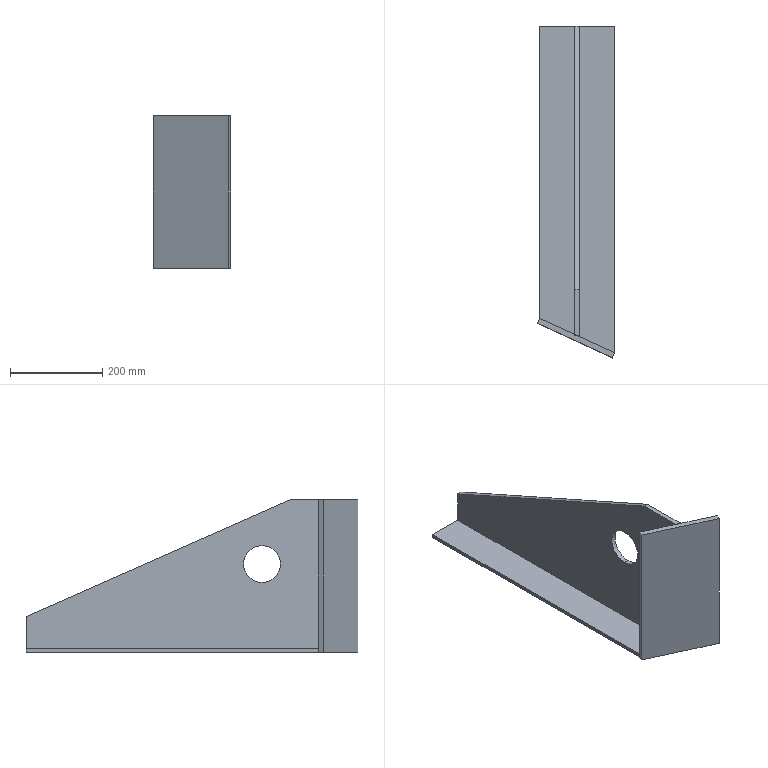Part | STEP file | Edge support_Default<As machined> | 3 solids | 21 faces | box 168.631 x 720.909 x 332 mm | volume 2997743 mm3 | plane 19 | cylinder 2 | commonest cylinder face diameters 80 x2
STEP:
#1=CARTESIAN_POINT('',(0.,0.,0.));
#2=DIRECTION('',(0.,0.,1.));
#3=DIRECTION('',(1.,0.,0.));
#4=AXIS2_PLACEMENT_3D('',#1,#2,#3);
#5=CARTESIAN_POINT('',(-81.815,0.,-4.));
#6=VERTEX_POINT('',#5);
#7=CARTESIAN_POINT('',(-81.815,-635.,-4.));
#8=VERTEX_POINT('',#7);
#9=CARTESIAN_POINT('',(-81.815,-635.,-4.));
#10=DIRECTION('',(0.,-1.,0.));
#11=VECTOR('',#10,1.);
#12=LINE('',#9,#11);
#13=CARTESIAN_POINT('',(-81.815,-635.,4.));
#14=DIRECTION('',(1.,0.,0.));
#15=DIRECTION('',(0.,0.,-1.));
#16=AXIS2_PLACEMENT_3D('',#13,#14,#15);
#17=PLANE('',#16);
#18=CARTESIAN_POINT('',(8.,0.));
#19=DIRECTION('',(0.,-1.));
#20=VECTOR('',#19,1.);
#21=LINE('',#18,#20);
#22=(GEOMETRIC_REPRESENTATION_CONTEXT(2)PARAMETRIC_REPRESENTATION_CONTEXT()REPRESENTATION_CONTEXT('',''));
#23=DEFINITIONAL_REPRESENTATION('',(#21),#22);
#24=PCURVE('',#17,#23);
#25=CARTESIAN_POINT('',(0.,0.,-4.));
#26=DIRECTION('',(0.,0.,-1.));
#27=DIRECTION('',(-1.,0.,0.));
#28=AXIS2_PLACEMENT_3D('',#25,#26,#27);
#29=PLANE('',#28);
#30=CARTESIAN_POINT('',(81.815,-635.));
#31=DIRECTION('',(0.,-1.));
#32=VECTOR('',#31,1.);
#33=LINE('',#30,#32);
#34=(GEOMETRIC_REPRESENTATION_CONTEXT(2)PARAMETRIC_REPRESENTATION_CONTEXT()REPRESENTATION_CONTEXT('',''));
#35=DEFINITIONAL_REPRESENTATION('',(#33),#34);
#36=PCURVE('',#29,#35);
#37=SURFACE_CURVE('',#12,(#24,#36),.PCURVE_S1.);
#38=EDGE_CURVE('',#6,#8,#37,.T.);
#39=ORIENTED_EDGE('',*,*,#38,.T.);
#40=CARTESIAN_POINT('',(-81.815,-635.,4.));
#41=VERTEX_POINT('',#40);
#42=CARTESIAN_POINT('',(-81.815,-635.,4.));
#43=DIRECTION('',(0.,0.,-1.));
#44=VECTOR('',#43,1.);
#45=LINE('',#42,#44);
#46=CARTESIAN_POINT('',(0.,0.));
#47=DIRECTION('',(1.,0.));
#48=VECTOR('',#47,1.);
#49=LINE('',#46,#48);
#50=(GEOMETRIC_REPRESENTATION_CONTEXT(2)PARAMETRIC_REPRESENTATION_CONTEXT()REPRESENTATION_CONTEXT('',''));
#51=DEFINITIONAL_REPRESENTATION('',(#49),#50);
#52=PCURVE('',#17,#51);
#53=CARTESIAN_POINT('',(81.815,-710.,4.));
#54=DIRECTION('',(0.4167,0.9091,0.));
#55=DIRECTION('',(-0.9091,0.4167,0.));
#56=AXIS2_PLACEMENT_3D('',#53,#54,#55);
#57=PLANE('',#56);
#58=CARTESIAN_POINT('',(180.,0.));
#59=DIRECTION('',(0.,-1.));
#60=VECTOR('',#59,1.);
#61=LINE('',#58,#60);
#62=(GEOMETRIC_REPRESENTATION_CONTEXT(2)PARAMETRIC_REPRESENTATION_CONTEXT()REPRESENTATION_CONTEXT('',''));
#63=DEFINITIONAL_REPRESENTATION('',(#61),#62);
#64=PCURVE('',#57,#63);
#65=SURFACE_CURVE('',#45,(#52,#64),.PCURVE_S1.);
#66=EDGE_CURVE('',#41,#8,#65,.T.);
#67=ORIENTED_EDGE('',*,*,#66,.F.);
#68=CARTESIAN_POINT('',(-81.815,0.,4.));
#69=VERTEX_POINT('',#68);
#70=CARTESIAN_POINT('',(-81.815,-635.,4.));
#71=DIRECTION('',(0.,-1.,0.));
#72=VECTOR('',#71,1.);
#73=LINE('',#70,#72);
#74=CARTESIAN_POINT('',(0.,0.));
#75=DIRECTION('',(0.,-1.));
#76=VECTOR('',#75,1.);
#77=LINE('',#74,#76);
#78=(GEOMETRIC_REPRESENTATION_CONTEXT(2)PARAMETRIC_REPRESENTATION_CONTEXT()REPRESENTATION_CONTEXT('',''));
#79=DEFINITIONAL_REPRESENTATION('',(#77),#78);
#80=PCURVE('',#17,#79);
#81=CARTESIAN_POINT('',(0.,0.,4.));
#82=DIRECTION('',(0.,0.,-1.));
#83=DIRECTION('',(-1.,0.,0.));
#84=AXIS2_PLACEMENT_3D('',#81,#82,#83);
#85=PLANE('',#84);
#86=CARTESIAN_POINT('',(81.815,-635.));
#87=DIRECTION('',(0.,-1.));
#88=VECTOR('',#87,1.);
#89=LINE('',#86,#88);
#90=(GEOMETRIC_REPRESENTATION_CONTEXT(2)PARAMETRIC_REPRESENTATION_CONTEXT()REPRESENTATION_CONTEXT('',''));
#91=DEFINITIONAL_REPRESENTATION('',(#89),#90);
#92=PCURVE('',#85,#91);
#93=SURFACE_CURVE('',#73,(#80,#92),.PCURVE_S1.);
#94=EDGE_CURVE('',#69,#41,#93,.T.);
#95=ORIENTED_EDGE('',*,*,#94,.F.);
#96=CARTESIAN_POINT('',(-81.815,0.,4.));
#97=DIRECTION('',(0.,0.,-1.));
#98=VECTOR('',#97,1.);
#99=LINE('',#96,#98);
#100=CARTESIAN_POINT('',(0.,635.));
#101=DIRECTION('',(1.,0.));
#102=VECTOR('',#101,1.);
#103=LINE('',#100,#102);
#104=(GEOMETRIC_REPRESENTATION_CONTEXT(2)PARAMETRIC_REPRESENTATION_CONTEXT()REPRESENTATION_CONTEXT('',''));
#105=DEFINITIONAL_REPRESENTATION('',(#103),#104);
#106=PCURVE('',#17,#105);
#107=CARTESIAN_POINT('',(-81.815,0.,4.));
#108=DIRECTION('',(0.,-1.,0.));
#109=DIRECTION('',(1.,0.,0.));
#110=AXIS2_PLACEMENT_3D('',#107,#108,#109);
#111=PLANE('',#110);
#112=CARTESIAN_POINT('',(0.,0.));
#113=DIRECTION('',(0.,-1.));
#114=VECTOR('',#113,1.);
#115=LINE('',#112,#114);
#116=(GEOMETRIC_REPRESENTATION_CONTEXT(2)PARAMETRIC_REPRESENTATION_CONTEXT()REPRESENTATION_CONTEXT('',''));
#117=DEFINITIONAL_REPRESENTATION('',(#115),#116);
#118=PCURVE('',#111,#117);
#119=SURFACE_CURVE('',#99,(#106,#118),.PCURVE_S1.);
#120=EDGE_CURVE('',#69,#6,#119,.T.);
#121=ORIENTED_EDGE('',*,*,#120,.T.);
#122=EDGE_LOOP('',(#39,#67,#95,#121));
#123=FACE_BOUND('',#122,.T.);
#124=ADVANCED_FACE('',(#123),#17,.F.);
#125=CARTESIAN_POINT('',(81.815,-710.,-4.));
#126=VERTEX_POINT('',#125);
#127=CARTESIAN_POINT('',(81.815,-710.,-4.));
#128=DIRECTION('',(0.9091,-0.4167,0.));
#129=VECTOR('',#128,1.);
#130=LINE('',#127,#129);
#131=CARTESIAN_POINT('',(0.,-8.));
#132=DIRECTION('',(-1.,0.));
#133=VECTOR('',#132,1.);
#134=LINE('',#131,#133);
#135=(GEOMETRIC_REPRESENTATION_CONTEXT(2)PARAMETRIC_REPRESENTATION_CONTEXT()REPRESENTATION_CONTEXT('',''));
#136=DEFINITIONAL_REPRESENTATION('',(#134),#135);
#137=PCURVE('',#57,#136);
#138=CARTESIAN_POINT('',(-81.815,-710.));
#139=DIRECTION('',(-0.9091,-0.4167));
#140=VECTOR('',#139,1.);
#141=LINE('',#138,#140);
#142=(GEOMETRIC_REPRESENTATION_CONTEXT(2)PARAMETRIC_REPRESENTATION_CONTEXT()REPRESENTATION_CONTEXT('',''));
#143=DEFINITIONAL_REPRESENTATION('',(#141),#142);
#144=PCURVE('',#29,#143);
#145=SURFACE_CURVE('',#130,(#137,#144),.PCURVE_S1.);
#146=EDGE_CURVE('',#8,#126,#145,.T.);
#147=ORIENTED_EDGE('',*,*,#146,.T.);
#148=CARTESIAN_POINT('',(81.815,-710.,4.));
#149=VERTEX_POINT('',#148);
#150=CARTESIAN_POINT('',(81.815,-710.,4.));
#151=DIRECTION('',(0.,0.,-1.));
#152=VECTOR('',#151,1.);
#153=LINE('',#150,#152);
#154=CARTESIAN_POINT('',(0.,0.));
#155=DIRECTION('',(0.,-1.));
#156=VECTOR('',#155,1.);
#157=LINE('',#154,#156);
#158=(GEOMETRIC_REPRESENTATION_CONTEXT(2)PARAMETRIC_REPRESENTATION_CONTEXT()REPRESENTATION_CONTEXT('',''));
#159=DEFINITIONAL_REPRESENTATION('',(#157),#158);
#160=PCURVE('',#57,#159);
#161=CARTESIAN_POINT('',(81.815,0.,4.));
#162=DIRECTION('',(-1.,0.,0.));
#163=DIRECTION('',(0.,0.,1.));
#164=AXIS2_PLACEMENT_3D('',#161,#162,#163);
#165=PLANE('',#164);
#166=CARTESIAN_POINT('',(0.,-710.));
#167=DIRECTION('',(-1.,0.));
#168=VECTOR('',#167,1.);
#169=LINE('',#166,#168);
#170=(GEOMETRIC_REPRESENTATION_CONTEXT(2)PARAMETRIC_REPRESENTATION_CONTEXT()REPRESENTATION_CONTEXT('',''));
#171=DEFINITIONAL_REPRESENTATION('',(#169),#170);
#172=PCURVE('',#165,#171);
#173=SURFACE_CURVE('',#153,(#160,#172),.PCURVE_S1.);
#174=EDGE_CURVE('',#149,#126,#173,.T.);
#175=ORIENTED_EDGE('',*,*,#174,.F.);
#176=CARTESIAN_POINT('',(81.815,-710.,4.));
#177=DIRECTION('',(0.9091,-0.4167,0.));
#178=VECTOR('',#177,1.);
#179=LINE('',#176,#178);
#180=CARTESIAN_POINT('',(0.,0.));
#181=DIRECTION('',(-1.,0.));
#182=VECTOR('',#181,1.);
#183=LINE('',#180,#182);
#184=(GEOMETRIC_REPRESENTATION_CONTEXT(2)PARAMETRIC_REPRESENTATION_CONTEXT()REPRESENTATION_CONTEXT('',''));
#185=DEFINITIONAL_REPRESENTATION('',(#183),#184);
#186=PCURVE('',#57,#185);
#187=CARTESIAN_POINT('',(-81.815,-710.));
#188=DIRECTION('',(-0.9091,-0.4167));
#189=VECTOR('',#188,1.);
#190=LINE('',#187,#189);
#191=(GEOMETRIC_REPRESENTATION_CONTEXT(2)PARAMETRIC_REPRESENTATION_CONTEXT()REPRESENTATION_CONTEXT('',''));
#192=DEFINITIONAL_REPRESENTATION('',(#190),#191);
#193=PCURVE('',#85,#192);
#194=SURFACE_CURVE('',#179,(#186,#193),.PCURVE_S1.);
#195=EDGE_CURVE('',#41,#149,#194,.T.);
#196=ORIENTED_EDGE('',*,*,#195,.F.);
#197=ORIENTED_EDGE('',*,*,#66,.T.);
#198=EDGE_LOOP('',(#147,#175,#196,#197));
#199=FACE_BOUND('',#198,.T.);
#200=ADVANCED_FACE('',(#199),#57,.F.);
#201=CARTESIAN_POINT('',(81.815,0.,-4.));
#202=VERTEX_POINT('',#201);
#203=CARTESIAN_POINT('',(81.815,0.,-4.));
#204=DIRECTION('',(0.,1.,0.));
#205=VECTOR('',#204,1.);
#206=LINE('',#203,#205);
#207=CARTESIAN_POINT('',(-8.,0.));
#208=DIRECTION('',(0.,1.));
#209=VECTOR('',#208,1.);
#210=LINE('',#207,#209);
#211=(GEOMETRIC_REPRESENTATION_CONTEXT(2)PARAMETRIC_REPRESENTATION_CONTEXT()REPRESENTATION_CONTEXT('',''));
#212=DEFINITIONAL_REPRESENTATION('',(#210),#211);
#213=PCURVE('',#165,#212);
#214=CARTESIAN_POINT('',(-81.815,0.));
#215=DIRECTION('',(0.,1.));
#216=VECTOR('',#215,1.);
#217=LINE('',#214,#216);
#218=(GEOMETRIC_REPRESENTATION_CONTEXT(2)PARAMETRIC_REPRESENTATION_CONTEXT()REPRESENTATION_CONTEXT('',''));
#219=DEFINITIONAL_REPRESENTATION('',(#217),#218);
#220=PCURVE('',#29,#219);
#221=SURFACE_CURVE('',#206,(#213,#220),.PCURVE_S1.);
#222=EDGE_CURVE('',#126,#202,#221,.T.);
#223=ORIENTED_EDGE('',*,*,#222,.T.);
#224=CARTESIAN_POINT('',(81.815,0.,4.));
#225=VERTEX_POINT('',#224);
#226=CARTESIAN_POINT('',(81.815,0.,4.));
#227=DIRECTION('',(0.,0.,-1.));
#228=VECTOR('',#227,1.);
#229=LINE('',#226,#228);
#230=CARTESIAN_POINT('',(0.,0.));
#231=DIRECTION('',(-1.,0.));
#232=VECTOR('',#231,1.);
#233=LINE('',#230,#232);
#234=(GEOMETRIC_REPRESENTATION_CONTEXT(2)PARAMETRIC_REPRESENTATION_CONTEXT()REPRESENTATION_CONTEXT('',''));
#235=DEFINITIONAL_REPRESENTATION('',(#233),#234);
#236=PCURVE('',#165,#235);
#237=CARTESIAN_POINT('',(163.631,0.));
#238=DIRECTION('',(0.,-1.));
#239=VECTOR('',#238,1.);
#240=LINE('',#237,#239);
#241=(GEOMETRIC_REPRESENTATION_CONTEXT(2)PARAMETRIC_REPRESENTATION_CONTEXT()REPRESENTATION_CONTEXT('',''));
#242=DEFINITIONAL_REPRESENTATION('',(#240),#241);
#243=PCURVE('',#111,#242);
#244=SURFACE_CURVE('',#229,(#236,#243),.PCURVE_S1.);
#245=EDGE_CURVE('',#225,#202,#244,.T.);
#246=ORIENTED_EDGE('',*,*,#245,.F.);
#247=CARTESIAN_POINT('',(81.815,0.,4.));
#248=DIRECTION('',(0.,1.,0.));
#249=VECTOR('',#248,1.);
#250=LINE('',#247,#249);
#251=CARTESIAN_POINT('',(0.,0.));
#252=DIRECTION('',(0.,1.));
#253=VECTOR('',#252,1.);
#254=LINE('',#251,#253);
#255=(GEOMETRIC_REPRESENTATION_CONTEXT(2)PARAMETRIC_REPRESENTATION_CONTEXT()REPRESENTATION_CONTEXT('',''));
#256=DEFINITIONAL_REPRESENTATION('',(#254),#255);
#257=PCURVE('',#165,#256);
#258=CARTESIAN_POINT('',(-81.815,0.));
#259=DIRECTION('',(0.,1.));
#260=VECTOR('',#259,1.);
#261=LINE('',#258,#260);
#262=(GEOMETRIC_REPRESENTATION_CONTEXT(2)PARAMETRIC_REPRESENTATION_CONTEXT()REPRESENTATION_CONTEXT('',''));
#263=DEFINITIONAL_REPRESENTATION('',(#261),#262);
#264=PCURVE('',#85,#263);
#265=SURFACE_CURVE('',#250,(#257,#264),.PCURVE_S1.);
#266=EDGE_CURVE('',#149,#225,#265,.T.);
#267=ORIENTED_EDGE('',*,*,#266,.F.);
#268=ORIENTED_EDGE('',*,*,#174,.T.);
#269=EDGE_LOOP('',(#223,#246,#267,#268));
#270=FACE_BOUND('',#269,.T.);
#271=ADVANCED_FACE('',(#270),#165,.F.);
#272=CARTESIAN_POINT('',(-81.815,0.,-4.));
#273=DIRECTION('',(-1.,0.,0.));
#274=VECTOR('',#273,1.);
#275=LINE('',#272,#274);
#276=CARTESIAN_POINT('',(0.,-8.));
#277=DIRECTION('',(-1.,0.));
#278=VECTOR('',#277,1.);
#279=LINE('',#276,#278);
#280=(GEOMETRIC_REPRESENTATION_CONTEXT(2)PARAMETRIC_REPRESENTATION_CONTEXT()REPRESENTATION_CONTEXT('',''));
#281=DEFINITIONAL_REPRESENTATION('',(#279),#280);
#282=PCURVE('',#111,#281);
#283=CARTESIAN_POINT('',(81.815,0.));
#284=DIRECTION('',(1.,0.));
#285=VECTOR('',#284,1.);
#286=LINE('',#283,#285);
#287=(GEOMETRIC_REPRESENTATION_CONTEXT(2)PARAMETRIC_REPRESENTATION_CONTEXT()REPRESENTATION_CONTEXT('',''));
#288=DEFINITIONAL_REPRESENTATION('',(#286),#287);
#289=PCURVE('',#29,#288);
#290=SURFACE_CURVE('',#275,(#282,#289),.PCURVE_S1.);
#291=EDGE_CURVE('',#202,#6,#290,.T.);
#292=ORIENTED_EDGE('',*,*,#291,.T.);
#293=ORIENTED_EDGE('',*,*,#120,.F.);
#294=CARTESIAN_POINT('',(-81.815,0.,4.));
#295=DIRECTION('',(-1.,0.,0.));
#296=VECTOR('',#295,1.);
#297=LINE('',#294,#296);
#298=CARTESIAN_POINT('',(0.,0.));
#299=DIRECTION('',(-1.,0.));
#300=VECTOR('',#299,1.);
#301=LINE('',#298,#300);
#302=(GEOMETRIC_REPRESENTATION_CONTEXT(2)PARAMETRIC_REPRESENTATION_CONTEXT()REPRESENTATION_CONTEXT('',''));
#303=DEFINITIONAL_REPRESENTATION('',(#301),#302);
#304=PCURVE('',#111,#303);
#305=CARTESIAN_POINT('',(81.815,0.));
#306=DIRECTION('',(1.,0.));
#307=VECTOR('',#306,1.);
#308=LINE('',#305,#307);
#309=(GEOMETRIC_REPRESENTATION_CONTEXT(2)PARAMETRIC_REPRESENTATION_CONTEXT()REPRESENTATION_CONTEXT('',''));
#310=DEFINITIONAL_REPRESENTATION('',(#308),#309);
#311=PCURVE('',#85,#310);
#312=SURFACE_CURVE('',#297,(#304,#311),.PCURVE_S1.);
#313=EDGE_CURVE('',#225,#69,#312,.T.);
#314=ORIENTED_EDGE('',*,*,#313,.F.);
#315=ORIENTED_EDGE('',*,*,#245,.T.);
#316=EDGE_LOOP('',(#292,#293,#314,#315));
#317=FACE_BOUND('',#316,.T.);
#318=ADVANCED_FACE('',(#317),#111,.F.);
#319=ORIENTED_EDGE('',*,*,#94,.T.);
#320=ORIENTED_EDGE('',*,*,#195,.T.);
#321=ORIENTED_EDGE('',*,*,#266,.T.);
#322=ORIENTED_EDGE('',*,*,#313,.T.);
#323=EDGE_LOOP('',(#319,#320,#321,#322));
#324=FACE_BOUND('',#323,.T.);
#325=ADVANCED_FACE('',(#324),#85,.F.);
#326=ORIENTED_EDGE('',*,*,#38,.F.);
#327=ORIENTED_EDGE('',*,*,#291,.F.);
#328=ORIENTED_EDGE('',*,*,#222,.F.);
#329=ORIENTED_EDGE('',*,*,#146,.F.);
#330=EDGE_LOOP('',(#326,#327,#328,#329));
#331=FACE_BOUND('',#330,.T.);
#332=ADVANCED_FACE('',(#331),#29,.T.);
#333=CLOSED_SHELL('',(#124,#200,#271,#318,#325,#332));
#334=MANIFOLD_SOLID_BREP('',#333);
#335=CARTESIAN_POINT('',(-81.815,-635.,-4.));
#336=VERTEX_POINT('',#335);
#337=CARTESIAN_POINT('',(-86.815,-645.909,-4.));
#338=VERTEX_POINT('',#337);
#339=CARTESIAN_POINT('',(-86.815,-645.909,-4.));
#340=DIRECTION('',(-0.4167,-0.9091,0.));
#341=VECTOR('',#340,1.);
#342=LINE('',#339,#341);
#343=CARTESIAN_POINT('',(-86.815,-645.909,328.));
#344=DIRECTION('',(0.9091,-0.4167,0.));
#345=DIRECTION('',(0.4167,0.9091,0.));
#346=AXIS2_PLACEMENT_3D('',#343,#344,#345);
#347=PLANE('',#346);
#348=CARTESIAN_POINT('',(0.,-332.));
#349=DIRECTION('',(-1.,0.));
#350=VECTOR('',#349,1.);
#351=LINE('',#348,#350);
#352=(GEOMETRIC_REPRESENTATION_CONTEXT(2)PARAMETRIC_REPRESENTATION_CONTEXT()REPRESENTATION_CONTEXT('',''));
#353=DEFINITIONAL_REPRESENTATION('',(#351),#352);
#354=PCURVE('',#347,#353);
#355=CARTESIAN_POINT('',(0.,0.,-4.));
#356=DIRECTION('',(0.,0.,-1.));
#357=DIRECTION('',(-1.,0.,0.));
#358=AXIS2_PLACEMENT_3D('',#355,#356,#357);
#359=PLANE('',#358);
#360=CARTESIAN_POINT('',(86.815,-645.909));
#361=DIRECTION('',(0.4167,-0.9091));
#362=VECTOR('',#361,1.);
#363=LINE('',#360,#362);
#364=(GEOMETRIC_REPRESENTATION_CONTEXT(2)PARAMETRIC_REPRESENTATION_CONTEXT()REPRESENTATION_CONTEXT('',''));
#365=DEFINITIONAL_REPRESENTATION('',(#363),#364);
#366=PCURVE('',#359,#365);
#367=SURFACE_CURVE('',#342,(#354,#366),.PCURVE_S1.);
#368=EDGE_CURVE('',#336,#338,#367,.T.);
#369=ORIENTED_EDGE('',*,*,#368,.T.);
#370=CARTESIAN_POINT('',(-86.815,-645.909,328.));
#371=VERTEX_POINT('',#370);
#372=CARTESIAN_POINT('',(-86.815,-645.909,328.));
#373=DIRECTION('',(0.,0.,-1.));
#374=VECTOR('',#373,1.);
#375=LINE('',#372,#374);
#376=CARTESIAN_POINT('',(0.,0.));
#377=DIRECTION('',(0.,-1.));
#378=VECTOR('',#377,1.);
#379=LINE('',#376,#378);
#380=(GEOMETRIC_REPRESENTATION_CONTEXT(2)PARAMETRIC_REPRESENTATION_CONTEXT()REPRESENTATION_CONTEXT('',''));
#381=DEFINITIONAL_REPRESENTATION('',(#379),#380);
#382=PCURVE('',#347,#381);
#383=CARTESIAN_POINT('',(76.815,-720.909,328.));
#384=DIRECTION('',(0.4167,0.9091,0.));
#385=DIRECTION('',(-0.9091,0.4167,0.));
#386=AXIS2_PLACEMENT_3D('',#383,#384,#385);
#387=PLANE('',#386);
#388=CARTESIAN_POINT('',(180.,0.));
#389=DIRECTION('',(0.,-1.));
#390=VECTOR('',#389,1.);
#391=LINE('',#388,#390);
#392=(GEOMETRIC_REPRESENTATION_CONTEXT(2)PARAMETRIC_REPRESENTATION_CONTEXT()REPRESENTATION_CONTEXT('',''));
#393=DEFINITIONAL_REPRESENTATION('',(#391),#392);
#394=PCURVE('',#387,#393);
#395=SURFACE_CURVE('',#375,(#382,#394),.PCURVE_S1.);
#396=EDGE_CURVE('',#371,#338,#395,.T.);
#397=ORIENTED_EDGE('',*,*,#396,.F.);
#398=CARTESIAN_POINT('',(-81.815,-635.,328.));
#399=VERTEX_POINT('',#398);
#400=CARTESIAN_POINT('',(-86.815,-645.909,328.));
#401=DIRECTION('',(-0.4167,-0.9091,0.));
#402=VECTOR('',#401,1.);
#403=LINE('',#400,#402);
#404=CARTESIAN_POINT('',(0.,0.));
#405=DIRECTION('',(-1.,0.));
#406=VECTOR('',#405,1.);
#407=LINE('',#404,#406);
#408=(GEOMETRIC_REPRESENTATION_CONTEXT(2)PARAMETRIC_REPRESENTATION_CONTEXT()REPRESENTATION_CONTEXT('',''));
#409=DEFINITIONAL_REPRESENTATION('',(#407),#408);
#410=PCURVE('',#347,#409);
#411=CARTESIAN_POINT('',(0.,0.,328.));
#412=DIRECTION('',(0.,0.,-1.));
#413=DIRECTION('',(-1.,0.,0.));
#414=AXIS2_PLACEMENT_3D('',#411,#412,#413);
#415=PLANE('',#414);
#416=CARTESIAN_POINT('',(86.815,-645.909));
#417=DIRECTION('',(0.4167,-0.9091));
#418=VECTOR('',#417,1.);
#419=LINE('',#416,#418);
#420=(GEOMETRIC_REPRESENTATION_CONTEXT(2)PARAMETRIC_REPRESENTATION_CONTEXT()REPRESENTATION_CONTEXT('',''));
#421=DEFINITIONAL_REPRESENTATION('',(#419),#420);
#422=PCURVE('',#415,#421);
#423=SURFACE_CURVE('',#403,(#410,#422),.PCURVE_S1.);
#424=EDGE_CURVE('',#399,#371,#423,.T.);
#425=ORIENTED_EDGE('',*,*,#424,.F.);
#426=CARTESIAN_POINT('',(-81.815,-635.,328.));
#427=DIRECTION('',(0.,0.,-1.));
#428=VECTOR('',#427,1.);
#429=LINE('',#426,#428);
#430=CARTESIAN_POINT('',(12.,0.));
#431=DIRECTION('',(0.,-1.));
#432=VECTOR('',#431,1.);
#433=LINE('',#430,#432);
#434=(GEOMETRIC_REPRESENTATION_CONTEXT(2)PARAMETRIC_REPRESENTATION_CONTEXT()REPRESENTATION_CONTEXT('',''));
#435=DEFINITIONAL_REPRESENTATION('',(#433),#434);
#436=PCURVE('',#347,#435);
#437=CARTESIAN_POINT('',(-81.815,-635.,328.));
#438=DIRECTION('',(-0.4167,-0.9091,0.));
#439=DIRECTION('',(0.9091,-0.4167,0.));
#440=AXIS2_PLACEMENT_3D('',#437,#438,#439);
#441=PLANE('',#440);
#442=CARTESIAN_POINT('',(0.,0.));
#443=DIRECTION('',(0.,-1.));
#444=VECTOR('',#443,1.);
#445=LINE('',#442,#444);
#446=(GEOMETRIC_REPRESENTATION_CONTEXT(2)PARAMETRIC_REPRESENTATION_CONTEXT()REPRESENTATION_CONTEXT('',''));
#447=DEFINITIONAL_REPRESENTATION('',(#445),#446);
#448=PCURVE('',#441,#447);
#449=SURFACE_CURVE('',#429,(#436,#448),.PCURVE_S1.);
#450=EDGE_CURVE('',#399,#336,#449,.T.);
#451=ORIENTED_EDGE('',*,*,#450,.T.);
#452=EDGE_LOOP('',(#369,#397,#425,#451));
#453=FACE_BOUND('',#452,.T.);
#454=ADVANCED_FACE('',(#453),#347,.F.);
#455=CARTESIAN_POINT('',(76.815,-720.909,-4.));
#456=VERTEX_POINT('',#455);
#457=CARTESIAN_POINT('',(76.815,-720.909,-4.));
#458=DIRECTION('',(0.9091,-0.4167,0.));
#459=VECTOR('',#458,1.);
#460=LINE('',#457,#459);
#461=CARTESIAN_POINT('',(0.,-332.));
#462=DIRECTION('',(-1.,0.));
#463=VECTOR('',#462,1.);
#464=LINE('',#461,#463);
#465=(GEOMETRIC_REPRESENTATION_CONTEXT(2)PARAMETRIC_REPRESENTATION_CONTEXT()REPRESENTATION_CONTEXT('',''));
#466=DEFINITIONAL_REPRESENTATION('',(#464),#465);
#467=PCURVE('',#387,#466);
#468=CARTESIAN_POINT('',(-76.815,-720.909));
#469=DIRECTION('',(-0.9091,-0.4167));
#470=VECTOR('',#469,1.);
#471=LINE('',#468,#470);
#472=(GEOMETRIC_REPRESENTATION_CONTEXT(2)PARAMETRIC_REPRESENTATION_CONTEXT()REPRESENTATION_CONTEXT('',''));
#473=DEFINITIONAL_REPRESENTATION('',(#471),#472);
#474=PCURVE('',#359,#473);
#475=SURFACE_CURVE('',#460,(#467,#474),.PCURVE_S1.);
#476=EDGE_CURVE('',#338,#456,#475,.T.);
#477=ORIENTED_EDGE('',*,*,#476,.T.);
#478=CARTESIAN_POINT('',(76.815,-720.909,328.));
#479=VERTEX_POINT('',#478);
#480=CARTESIAN_POINT('',(76.815,-720.909,328.));
#481=DIRECTION('',(0.,0.,-1.));
#482=VECTOR('',#481,1.);
#483=LINE('',#480,#482);
#484=CARTESIAN_POINT('',(0.,0.));
#485=DIRECTION('',(0.,-1.));
#486=VECTOR('',#485,1.);
#487=LINE('',#484,#486);
#488=(GEOMETRIC_REPRESENTATION_CONTEXT(2)PARAMETRIC_REPRESENTATION_CONTEXT()REPRESENTATION_CONTEXT('',''));
#489=DEFINITIONAL_REPRESENTATION('',(#487),#488);
#490=PCURVE('',#387,#489);
#491=CARTESIAN_POINT('',(81.815,-710.,328.));
#492=DIRECTION('',(-0.9091,0.4167,0.));
#493=DIRECTION('',(-0.4167,-0.9091,0.));
#494=AXIS2_PLACEMENT_3D('',#491,#492,#493);
#495=PLANE('',#494);
#496=CARTESIAN_POINT('',(12.,0.));
#497=DIRECTION('',(0.,-1.));
#498=VECTOR('',#497,1.);
#499=LINE('',#496,#498);
#500=(GEOMETRIC_REPRESENTATION_CONTEXT(2)PARAMETRIC_REPRESENTATION_CONTEXT()REPRESENTATION_CONTEXT('',''));
#501=DEFINITIONAL_REPRESENTATION('',(#499),#500);
#502=PCURVE('',#495,#501);
#503=SURFACE_CURVE('',#483,(#490,#502),.PCURVE_S1.);
#504=EDGE_CURVE('',#479,#456,#503,.T.);
#505=ORIENTED_EDGE('',*,*,#504,.F.);
#506=CARTESIAN_POINT('',(76.815,-720.909,328.));
#507=DIRECTION('',(0.9091,-0.4167,0.));
#508=VECTOR('',#507,1.);
#509=LINE('',#506,#508);
#510=CARTESIAN_POINT('',(0.,0.));
#511=DIRECTION('',(-1.,0.));
#512=VECTOR('',#511,1.);
#513=LINE('',#510,#512);
#514=(GEOMETRIC_REPRESENTATION_CONTEXT(2)PARAMETRIC_REPRESENTATION_CONTEXT()REPRESENTATION_CONTEXT('',''));
#515=DEFINITIONAL_REPRESENTATION('',(#513),#514);
#516=PCURVE('',#387,#515);
#517=CARTESIAN_POINT('',(-76.815,-720.909));
#518=DIRECTION('',(-0.9091,-0.4167));
#519=VECTOR('',#518,1.);
#520=LINE('',#517,#519);
#521=(GEOMETRIC_REPRESENTATION_CONTEXT(2)PARAMETRIC_REPRESENTATION_CONTEXT()REPRESENTATION_CONTEXT('',''));
#522=DEFINITIONAL_REPRESENTATION('',(#520),#521);
#523=PCURVE('',#415,#522);
#524=SURFACE_CURVE('',#509,(#516,#523),.PCURVE_S1.);
#525=EDGE_CURVE('',#371,#479,#524,.T.);
#526=ORIENTED_EDGE('',*,*,#525,.F.);
#527=ORIENTED_EDGE('',*,*,#396,.T.);
#528=EDGE_LOOP('',(#477,#505,#526,#527));
#529=FACE_BOUND('',#528,.T.);
#530=ADVANCED_FACE('',(#529),#387,.F.);
#531=CARTESIAN_POINT('',(81.815,-710.,-4.));
#532=VERTEX_POINT('',#531);
#533=CARTESIAN_POINT('',(81.815,-710.,-4.));
#534=DIRECTION('',(0.4167,0.9091,0.));
#535=VECTOR('',#534,1.);
#536=LINE('',#533,#535);
#537=CARTESIAN_POINT('',(0.,-332.));
#538=DIRECTION('',(-1.,0.));
#539=VECTOR('',#538,1.);
#540=LINE('',#537,#539);
#541=(GEOMETRIC_REPRESENTATION_CONTEXT(2)PARAMETRIC_REPRESENTATION_CONTEXT()REPRESENTATION_CONTEXT('',''));
#542=DEFINITIONAL_REPRESENTATION('',(#540),#541);
#543=PCURVE('',#495,#542);
#544=CARTESIAN_POINT('',(-81.815,-710.));
#545=DIRECTION('',(-0.4167,0.9091));
#546=VECTOR('',#545,1.);
#547=LINE('',#544,#546);
#548=(GEOMETRIC_REPRESENTATION_CONTEXT(2)PARAMETRIC_REPRESENTATION_CONTEXT()REPRESENTATION_CONTEXT('',''));
#549=DEFINITIONAL_REPRESENTATION('',(#547),#548);
#550=PCURVE('',#359,#549);
#551=SURFACE_CURVE('',#536,(#543,#550),.PCURVE_S1.);
#552=EDGE_CURVE('',#456,#532,#551,.T.);
#553=ORIENTED_EDGE('',*,*,#552,.T.);
#554=CARTESIAN_POINT('',(81.815,-710.,328.));
#555=VERTEX_POINT('',#554);
#556=CARTESIAN_POINT('',(81.815,-710.,328.));
#557=DIRECTION('',(0.,0.,-1.));
#558=VECTOR('',#557,1.);
#559=LINE('',#556,#558);
#560=CARTESIAN_POINT('',(0.,0.));
#561=DIRECTION('',(0.,-1.));
#562=VECTOR('',#561,1.);
#563=LINE('',#560,#562);
#564=(GEOMETRIC_REPRESENTATION_CONTEXT(2)PARAMETRIC_REPRESENTATION_CONTEXT()REPRESENTATION_CONTEXT('',''));
#565=DEFINITIONAL_REPRESENTATION('',(#563),#564);
#566=PCURVE('',#495,#565);
#567=CARTESIAN_POINT('',(180.,0.));
#568=DIRECTION('',(0.,-1.));
#569=VECTOR('',#568,1.);
#570=LINE('',#567,#569);
#571=(GEOMETRIC_REPRESENTATION_CONTEXT(2)PARAMETRIC_REPRESENTATION_CONTEXT()REPRESENTATION_CONTEXT('',''));
#572=DEFINITIONAL_REPRESENTATION('',(#570),#571);
#573=PCURVE('',#441,#572);
#574=SURFACE_CURVE('',#559,(#566,#573),.PCURVE_S1.);
#575=EDGE_CURVE('',#555,#532,#574,.T.);
#576=ORIENTED_EDGE('',*,*,#575,.F.);
#577=CARTESIAN_POINT('',(81.815,-710.,328.));
#578=DIRECTION('',(0.4167,0.9091,0.));
#579=VECTOR('',#578,1.);
#580=LINE('',#577,#579);
#581=CARTESIAN_POINT('',(0.,0.));
#582=DIRECTION('',(-1.,0.));
#583=VECTOR('',#582,1.);
#584=LINE('',#581,#583);
#585=(GEOMETRIC_REPRESENTATION_CONTEXT(2)PARAMETRIC_REPRESENTATION_CONTEXT()REPRESENTATION_CONTEXT('',''));
#586=DEFINITIONAL_REPRESENTATION('',(#584),#585);
#587=PCURVE('',#495,#586);
#588=CARTESIAN_POINT('',(-81.815,-710.));
#589=DIRECTION('',(-0.4167,0.9091));
#590=VECTOR('',#589,1.);
#591=LINE('',#588,#590);
#592=(GEOMETRIC_REPRESENTATION_CONTEXT(2)PARAMETRIC_REPRESENTATION_CONTEXT()REPRESENTATION_CONTEXT('',''));
#593=DEFINITIONAL_REPRESENTATION('',(#591),#592);
#594=PCURVE('',#415,#593);
#595=SURFACE_CURVE('',#580,(#587,#594),.PCURVE_S1.);
#596=EDGE_CURVE('',#479,#555,#595,.T.);
#597=ORIENTED_EDGE('',*,*,#596,.F.);
#598=ORIENTED_EDGE('',*,*,#504,.T.);
#599=EDGE_LOOP('',(#553,#576,#597,#598));
#600=FACE_BOUND('',#599,.T.);
#601=ADVANCED_FACE('',(#600),#495,.F.);
#602=CARTESIAN_POINT('',(-81.815,-635.,-4.));
#603=DIRECTION('',(-0.9091,0.4167,0.));
#604=VECTOR('',#603,1.);
#605=LINE('',#602,#604);
#606=CARTESIAN_POINT('',(0.,-332.));
#607=DIRECTION('',(-1.,0.));
#608=VECTOR('',#607,1.);
#609=LINE('',#606,#608);
#610=(GEOMETRIC_REPRESENTATION_CONTEXT(2)PARAMETRIC_REPRESENTATION_CONTEXT()REPRESENTATION_CONTEXT('',''));
#611=DEFINITIONAL_REPRESENTATION('',(#609),#610);
#612=PCURVE('',#441,#611);
#613=CARTESIAN_POINT('',(81.815,-635.));
#614=DIRECTION('',(0.9091,0.4167));
#615=VECTOR('',#614,1.);
#616=LINE('',#613,#615);
#617=(GEOMETRIC_REPRESENTATION_CONTEXT(2)PARAMETRIC_REPRESENTATION_CONTEXT()REPRESENTATION_CONTEXT('',''));
#618=DEFINITIONAL_REPRESENTATION('',(#616),#617);
#619=PCURVE('',#359,#618);
#620=SURFACE_CURVE('',#605,(#612,#619),.PCURVE_S1.);
#621=EDGE_CURVE('',#532,#336,#620,.T.);
#622=ORIENTED_EDGE('',*,*,#621,.T.);
#623=ORIENTED_EDGE('',*,*,#450,.F.);
#624=CARTESIAN_POINT('',(-81.815,-635.,328.));
#625=DIRECTION('',(-0.9091,0.4167,0.));
#626=VECTOR('',#625,1.);
#627=LINE('',#624,#626);
#628=CARTESIAN_POINT('',(0.,0.));
#629=DIRECTION('',(-1.,0.));
#630=VECTOR('',#629,1.);
#631=LINE('',#628,#630);
#632=(GEOMETRIC_REPRESENTATION_CONTEXT(2)PARAMETRIC_REPRESENTATION_CONTEXT()REPRESENTATION_CONTEXT('',''));
#633=DEFINITIONAL_REPRESENTATION('',(#631),#632);
#634=PCURVE('',#441,#633);
#635=CARTESIAN_POINT('',(81.815,-635.));
#636=DIRECTION('',(0.9091,0.4167));
#637=VECTOR('',#636,1.);
#638=LINE('',#635,#637);
#639=(GEOMETRIC_REPRESENTATION_CONTEXT(2)PARAMETRIC_REPRESENTATION_CONTEXT()REPRESENTATION_CONTEXT('',''));
#640=DEFINITIONAL_REPRESENTATION('',(#638),#639);
#641=PCURVE('',#415,#640);
#642=SURFACE_CURVE('',#627,(#634,#641),.PCURVE_S1.);
#643=EDGE_CURVE('',#555,#399,#642,.T.);
#644=ORIENTED_EDGE('',*,*,#643,.F.);
#645=ORIENTED_EDGE('',*,*,#575,.T.);
#646=EDGE_LOOP('',(#622,#623,#644,#645));
#647=FACE_BOUND('',#646,.T.);
#648=ADVANCED_FACE('',(#647),#441,.F.);
#649=ORIENTED_EDGE('',*,*,#424,.T.);
#650=ORIENTED_EDGE('',*,*,#525,.T.);
#651=ORIENTED_EDGE('',*,*,#596,.T.);
#652=ORIENTED_EDGE('',*,*,#643,.T.);
#653=EDGE_LOOP('',(#649,#650,#651,#652));
#654=FACE_BOUND('',#653,.T.);
#655=ADVANCED_FACE('',(#654),#415,.F.);
#656=ORIENTED_EDGE('',*,*,#368,.F.);
#657=ORIENTED_EDGE('',*,*,#621,.F.);
#658=ORIENTED_EDGE('',*,*,#552,.F.);
#659=ORIENTED_EDGE('',*,*,#476,.F.);
#660=EDGE_LOOP('',(#656,#657,#658,#659));
#661=FACE_BOUND('',#660,.T.);
#662=ADVANCED_FACE('',(#661),#359,.T.);
#663=CLOSED_SHELL('',(#454,#530,#601,#648,#655,#662));
#664=MANIFOLD_SOLID_BREP('',#663);
#665=CARTESIAN_POINT('',(5.,-512.5,228.));
#666=VERTEX_POINT('',#665);
#667=CARTESIAN_POINT('',(-5.,-512.5,228.));
#668=VERTEX_POINT('',#667);
#669=CARTESIAN_POINT('',(5.,-512.5,228.));
#670=DIRECTION('',(-1.,0.,0.));
#671=VECTOR('',#670,1.);
#672=LINE('',#669,#671);
#673=CARTESIAN_POINT('',(5.,-512.5,188.));
#674=DIRECTION('',(-1.,0.,0.));
#675=DIRECTION('',(0.,0.,1.));
#676=AXIS2_PLACEMENT_3D('',#673,#674,#675);
#677=CYLINDRICAL_SURFACE('',#676,40.);
#678=CARTESIAN_POINT('',(6.283,0.));
#679=DIRECTION('',(0.,1.));
#680=VECTOR('',#679,1.);
#681=LINE('',#678,#680);
#682=(GEOMETRIC_REPRESENTATION_CONTEXT(2)PARAMETRIC_REPRESENTATION_CONTEXT()REPRESENTATION_CONTEXT('',''));
#683=DEFINITIONAL_REPRESENTATION('',(#681),#682);
#684=PCURVE('',#677,#683);
#685=CARTESIAN_POINT('',(5.,-512.5,188.));
#686=DIRECTION('',(-1.,0.,0.));
#687=DIRECTION('',(0.,0.,1.));
#688=AXIS2_PLACEMENT_3D('',#685,#686,#687);
#689=CYLINDRICAL_SURFACE('',#688,40.);
#690=CARTESIAN_POINT('',(0.,0.));
#691=DIRECTION('',(0.,1.));
#692=VECTOR('',#691,1.);
#693=LINE('',#690,#692);
#694=(GEOMETRIC_REPRESENTATION_CONTEXT(2)PARAMETRIC_REPRESENTATION_CONTEXT()REPRESENTATION_CONTEXT('',''));
#695=DEFINITIONAL_REPRESENTATION('',(#693),#694);
#696=PCURVE('',#689,#695);
#697=SURFACE_CURVE('',#672,(#684,#696),.PCURVE_S1.);
#698=EDGE_CURVE('',#666,#668,#697,.T.);
#699=ORIENTED_EDGE('',*,*,#698,.T.);
#700=CARTESIAN_POINT('',(-5.,-512.5,148.));
#701=VERTEX_POINT('',#700);
#702=CARTESIAN_POINT('',(-5.,-512.5,188.));
#703=DIRECTION('',(1.,0.,0.));
#704=DIRECTION('',(0.,0.,-1.));
#705=AXIS2_PLACEMENT_3D('',#702,#703,#704);
#706=CIRCLE('',#705,40.);
#707=CARTESIAN_POINT('',(9.425,10.));
#708=DIRECTION('',(-1.,0.));
#709=VECTOR('',#708,1.);
#710=LINE('',#707,#709);
#711=(GEOMETRIC_REPRESENTATION_CONTEXT(2)PARAMETRIC_REPRESENTATION_CONTEXT()REPRESENTATION_CONTEXT('',''));
#712=DEFINITIONAL_REPRESENTATION('',(#710),#711);
#713=PCURVE('',#677,#712);
#714=CARTESIAN_POINT('',(-5.,0.,0.));
#715=DIRECTION('',(1.,0.,0.));
#716=DIRECTION('',(0.,0.,-1.));
#717=AXIS2_PLACEMENT_3D('',#714,#715,#716);
#718=PLANE('',#717);
#719=CARTESIAN_POINT('',(-188.,-512.5));
#720=DIRECTION('',(1.,0.));
#721=AXIS2_PLACEMENT_2D('',#719,#720);
#722=CIRCLE('',#721,40.);
#723=(GEOMETRIC_REPRESENTATION_CONTEXT(2)PARAMETRIC_REPRESENTATION_CONTEXT()REPRESENTATION_CONTEXT('',''));
#724=DEFINITIONAL_REPRESENTATION('',(#722),#723);
#725=PCURVE('',#718,#724);
#726=SURFACE_CURVE('',#706,(#713,#725),.PCURVE_S1.);
#727=EDGE_CURVE('',#668,#701,#726,.T.);
#728=ORIENTED_EDGE('',*,*,#727,.T.);
#729=CARTESIAN_POINT('',(5.,-512.5,148.));
#730=VERTEX_POINT('',#729);
#731=CARTESIAN_POINT('',(5.,-512.5,148.));
#732=DIRECTION('',(-1.,0.,0.));
#733=VECTOR('',#732,1.);
#734=LINE('',#731,#733);
#735=CARTESIAN_POINT('',(3.142,0.));
#736=DIRECTION('',(0.,1.));
#737=VECTOR('',#736,1.);
#738=LINE('',#735,#737);
#739=(GEOMETRIC_REPRESENTATION_CONTEXT(2)PARAMETRIC_REPRESENTATION_CONTEXT()REPRESENTATION_CONTEXT('',''));
#740=DEFINITIONAL_REPRESENTATION('',(#738),#739);
#741=PCURVE('',#677,#740);
#742=CARTESIAN_POINT('',(3.142,0.));
#743=DIRECTION('',(0.,1.));
#744=VECTOR('',#743,1.);
#745=LINE('',#742,#744);
#746=(GEOMETRIC_REPRESENTATION_CONTEXT(2)PARAMETRIC_REPRESENTATION_CONTEXT()REPRESENTATION_CONTEXT('',''));
#747=DEFINITIONAL_REPRESENTATION('',(#745),#746);
#748=PCURVE('',#689,#747);
#749=SURFACE_CURVE('',#734,(#741,#748),.PCURVE_S1.);
#750=EDGE_CURVE('',#730,#701,#749,.T.);
#751=ORIENTED_EDGE('',*,*,#750,.F.);
#752=CARTESIAN_POINT('',(5.,-512.5,188.));
#753=DIRECTION('',(1.,0.,0.));
#754=DIRECTION('',(0.,0.,-1.));
#755=AXIS2_PLACEMENT_3D('',#752,#753,#754);
#756=CIRCLE('',#755,40.);
#757=CARTESIAN_POINT('',(9.425,0.));
#758=DIRECTION('',(-1.,0.));
#759=VECTOR('',#758,1.);
#760=LINE('',#757,#759);
#761=(GEOMETRIC_REPRESENTATION_CONTEXT(2)PARAMETRIC_REPRESENTATION_CONTEXT()REPRESENTATION_CONTEXT('',''));
#762=DEFINITIONAL_REPRESENTATION('',(#760),#761);
#763=PCURVE('',#677,#762);
#764=CARTESIAN_POINT('',(5.,0.,0.));
#765=DIRECTION('',(1.,0.,0.));
#766=DIRECTION('',(0.,0.,-1.));
#767=AXIS2_PLACEMENT_3D('',#764,#765,#766);
#768=PLANE('',#767);
#769=CARTESIAN_POINT('',(-188.,-512.5));
#770=DIRECTION('',(1.,0.));
#771=AXIS2_PLACEMENT_2D('',#769,#770);
#772=CIRCLE('',#771,40.);
#773=(GEOMETRIC_REPRESENTATION_CONTEXT(2)PARAMETRIC_REPRESENTATION_CONTEXT()REPRESENTATION_CONTEXT('',''));
#774=DEFINITIONAL_REPRESENTATION('',(#772),#773);
#775=PCURVE('',#768,#774);
#776=SURFACE_CURVE('',#756,(#763,#775),.PCURVE_S1.);
#777=EDGE_CURVE('',#666,#730,#776,.T.);
#778=ORIENTED_EDGE('',*,*,#777,.F.);
#779=EDGE_LOOP('',(#699,#728,#751,#778));
#780=FACE_BOUND('',#779,.F.);
#781=ADVANCED_FACE('',(#780),#677,.F.);
#782=CARTESIAN_POINT('',(5.,-672.5,4.));
#783=VERTEX_POINT('',#782);
#784=CARTESIAN_POINT('',(5.,0.,4.));
#785=VERTEX_POINT('',#784);
#786=CARTESIAN_POINT('',(5.,-672.5,4.));
#787=DIRECTION('',(0.,1.,0.));
#788=VECTOR('',#787,1.);
#789=LINE('',#786,#788);
#790=CARTESIAN_POINT('',(-4.,-672.5));
#791=DIRECTION('',(0.,1.));
#792=VECTOR('',#791,1.);
#793=LINE('',#790,#792);
#794=(GEOMETRIC_REPRESENTATION_CONTEXT(2)PARAMETRIC_REPRESENTATION_CONTEXT()REPRESENTATION_CONTEXT('',''));
#795=DEFINITIONAL_REPRESENTATION('',(#793),#794);
#796=PCURVE('',#768,#795);
#797=CARTESIAN_POINT('',(5.,-672.5,4.));
#798=DIRECTION('',(0.,0.,1.));
#799=DIRECTION('',(1.,0.,0.));
#800=AXIS2_PLACEMENT_3D('',#797,#798,#799);
#801=PLANE('',#800);
#802=CARTESIAN_POINT('',(0.,0.));
#803=DIRECTION('',(0.,1.));
#804=VECTOR('',#803,1.);
#805=LINE('',#802,#804);
#806=(GEOMETRIC_REPRESENTATION_CONTEXT(2)PARAMETRIC_REPRESENTATION_CONTEXT()REPRESENTATION_CONTEXT('',''));
#807=DEFINITIONAL_REPRESENTATION('',(#805),#806);
#808=PCURVE('',#801,#807);
#809=SURFACE_CURVE('',#789,(#796,#808),.PCURVE_S1.);
#810=EDGE_CURVE('',#783,#785,#809,.T.);
#811=ORIENTED_EDGE('',*,*,#810,.T.);
#812=CARTESIAN_POINT('',(5.,0.,74.));
#813=VERTEX_POINT('',#812);
#814=CARTESIAN_POINT('',(5.,0.,4.));
#815=DIRECTION('',(0.,0.,1.));
#816=VECTOR('',#815,1.);
#817=LINE('',#814,#816);
#818=CARTESIAN_POINT('',(-4.,0.));
#819=DIRECTION('',(-1.,0.));
#820=VECTOR('',#819,1.);
#821=LINE('',#818,#820);
#822=(GEOMETRIC_REPRESENTATION_CONTEXT(2)PARAMETRIC_REPRESENTATION_CONTEXT()REPRESENTATION_CONTEXT('',''));
#823=DEFINITIONAL_REPRESENTATION('',(#821),#822);
#824=PCURVE('',#768,#823);
#825=CARTESIAN_POINT('',(5.,0.,4.));
#826=DIRECTION('',(0.,-1.,0.));
#827=DIRECTION('',(0.,0.,-1.));
#828=AXIS2_PLACEMENT_3D('',#825,#826,#827);
#829=PLANE('',#828);
#830=CARTESIAN_POINT('',(0.,0.));
#831=DIRECTION('',(-1.,0.));
#832=VECTOR('',#831,1.);
#833=LINE('',#830,#832);
#834=(GEOMETRIC_REPRESENTATION_CONTEXT(2)PARAMETRIC_REPRESENTATION_CONTEXT()REPRESENTATION_CONTEXT('',''));
#835=DEFINITIONAL_REPRESENTATION('',(#833),#834);
#836=PCURVE('',#829,#835);
#837=SURFACE_CURVE('',#817,(#824,#836),.PCURVE_S1.);
#838=EDGE_CURVE('',#785,#813,#837,.T.);
#839=ORIENTED_EDGE('',*,*,#838,.T.);
#840=CARTESIAN_POINT('',(5.,-573.5,328.));
#841=VERTEX_POINT('',#840);
#842=CARTESIAN_POINT('',(5.,0.,74.));
#843=DIRECTION('',(0.,-0.9143,0.405));
#844=VECTOR('',#843,1.);
#845=LINE('',#842,#844);
#846=CARTESIAN_POINT('',(-74.,0.));
#847=DIRECTION('',(-0.405,-0.9143));
#848=VECTOR('',#847,1.);
#849=LINE('',#846,#848);
#850=(GEOMETRIC_REPRESENTATION_CONTEXT(2)PARAMETRIC_REPRESENTATION_CONTEXT()REPRESENTATION_CONTEXT('',''));
#851=DEFINITIONAL_REPRESENTATION('',(#849),#850);
#852=PCURVE('',#768,#851);
#853=CARTESIAN_POINT('',(5.,0.,74.));
#854=DIRECTION('',(0.,-0.405,-0.9143));
#855=DIRECTION('',(0.,0.9143,-0.405));
#856=AXIS2_PLACEMENT_3D('',#853,#854,#855);
#857=PLANE('',#856);
#858=CARTESIAN_POINT('',(0.,0.));
#859=DIRECTION('',(-1.,0.));
#860=VECTOR('',#859,1.);
#861=LINE('',#858,#860);
#862=(GEOMETRIC_REPRESENTATION_CONTEXT(2)PARAMETRIC_REPRESENTATION_CONTEXT()REPRESENTATION_CONTEXT('',''));
#863=DEFINITIONAL_REPRESENTATION('',(#861),#862);
#864=PCURVE('',#857,#863);
#865=SURFACE_CURVE('',#845,(#852,#864),.PCURVE_S1.);
#866=EDGE_CURVE('',#813,#841,#865,.T.);
#867=ORIENTED_EDGE('',*,*,#866,.T.);
#868=CARTESIAN_POINT('',(5.,-672.5,328.));
#869=VERTEX_POINT('',#868);
#870=CARTESIAN_POINT('',(5.,-573.5,328.));
#871=DIRECTION('',(0.,-1.,0.));
#872=VECTOR('',#871,1.);
#873=LINE('',#870,#872);
#874=CARTESIAN_POINT('',(-328.,-573.5));
#875=DIRECTION('',(0.,-1.));
#876=VECTOR('',#875,1.);
#877=LINE('',#874,#876);
#878=(GEOMETRIC_REPRESENTATION_CONTEXT(2)PARAMETRIC_REPRESENTATION_CONTEXT()REPRESENTATION_CONTEXT('',''));
#879=DEFINITIONAL_REPRESENTATION('',(#877),#878);
#880=PCURVE('',#768,#879);
#881=CARTESIAN_POINT('',(5.,-573.5,328.));
#882=DIRECTION('',(0.,0.,-1.));
#883=DIRECTION('',(-1.,0.,0.));
#884=AXIS2_PLACEMENT_3D('',#881,#882,#883);
#885=PLANE('',#884);
#886=CARTESIAN_POINT('',(0.,0.));
#887=DIRECTION('',(0.,-1.));
#888=VECTOR('',#887,1.);
#889=LINE('',#886,#888);
#890=(GEOMETRIC_REPRESENTATION_CONTEXT(2)PARAMETRIC_REPRESENTATION_CONTEXT()REPRESENTATION_CONTEXT('',''));
#891=DEFINITIONAL_REPRESENTATION('',(#889),#890);
#892=PCURVE('',#885,#891);
#893=SURFACE_CURVE('',#873,(#880,#892),.PCURVE_S1.);
#894=EDGE_CURVE('',#841,#869,#893,.T.);
#895=ORIENTED_EDGE('',*,*,#894,.T.);
#896=CARTESIAN_POINT('',(5.,-672.5,328.));
#897=DIRECTION('',(0.,0.,-1.));
#898=VECTOR('',#897,1.);
#899=LINE('',#896,#898);
#900=CARTESIAN_POINT('',(-328.,-672.5));
#901=DIRECTION('',(1.,0.));
#902=VECTOR('',#901,1.);
#903=LINE('',#900,#902);
#904=(GEOMETRIC_REPRESENTATION_CONTEXT(2)PARAMETRIC_REPRESENTATION_CONTEXT()REPRESENTATION_CONTEXT('',''));
#905=DEFINITIONAL_REPRESENTATION('',(#903),#904);
#906=PCURVE('',#768,#905);
#907=CARTESIAN_POINT('',(5.,-672.5,328.));
#908=DIRECTION('',(0.,1.,0.));
#909=DIRECTION('',(0.,0.,1.));
#910=AXIS2_PLACEMENT_3D('',#907,#908,#909);
#911=PLANE('',#910);
#912=CARTESIAN_POINT('',(0.,0.));
#913=DIRECTION('',(-1.,0.));
#914=VECTOR('',#913,1.);
#915=LINE('',#912,#914);
#916=(GEOMETRIC_REPRESENTATION_CONTEXT(2)PARAMETRIC_REPRESENTATION_CONTEXT()REPRESENTATION_CONTEXT('',''));
#917=DEFINITIONAL_REPRESENTATION('',(#915),#916);
#918=PCURVE('',#911,#917);
#919=SURFACE_CURVE('',#899,(#906,#918),.PCURVE_S1.);
#920=EDGE_CURVE('',#869,#783,#919,.T.);
#921=ORIENTED_EDGE('',*,*,#920,.T.);
#922=EDGE_LOOP('',(#811,#839,#867,#895,#921));
#923=FACE_BOUND('',#922,.T.);
#924=ORIENTED_EDGE('',*,*,#777,.F.);
#925=CARTESIAN_POINT('',(5.,-512.5,188.));
#926=DIRECTION('',(1.,0.,0.));
#927=DIRECTION('',(0.,0.,-1.));
#928=AXIS2_PLACEMENT_3D('',#925,#926,#927);
#929=CIRCLE('',#928,40.);
#930=CARTESIAN_POINT('',(-188.,-512.5));
#931=DIRECTION('',(1.,0.));
#932=AXIS2_PLACEMENT_2D('',#930,#931);
#933=CIRCLE('',#932,40.);
#934=(GEOMETRIC_REPRESENTATION_CONTEXT(2)PARAMETRIC_REPRESENTATION_CONTEXT()REPRESENTATION_CONTEXT('',''));
#935=DEFINITIONAL_REPRESENTATION('',(#933),#934);
#936=PCURVE('',#768,#935);
#937=CARTESIAN_POINT('',(3.142,0.));
#938=DIRECTION('',(-1.,0.));
#939=VECTOR('',#938,1.);
#940=LINE('',#937,#939);
#941=(GEOMETRIC_REPRESENTATION_CONTEXT(2)PARAMETRIC_REPRESENTATION_CONTEXT()REPRESENTATION_CONTEXT('',''));
#942=DEFINITIONAL_REPRESENTATION('',(#940),#941);
#943=PCURVE('',#689,#942);
#944=SURFACE_CURVE('',#929,(#936,#943),.PCURVE_S1.);
#945=EDGE_CURVE('',#730,#666,#944,.T.);
#946=ORIENTED_EDGE('',*,*,#945,.F.);
#947=EDGE_LOOP('',(#924,#946));
#948=FACE_BOUND('',#947,.T.);
#949=ADVANCED_FACE('',(#923,#948),#768,.T.);
#950=CARTESIAN_POINT('',(-5.,-672.5,4.));
#951=VERTEX_POINT('',#950);
#952=CARTESIAN_POINT('',(-5.,0.,4.));
#953=VERTEX_POINT('',#952);
#954=CARTESIAN_POINT('',(-5.,-672.5,4.));
#955=DIRECTION('',(0.,1.,0.));
#956=VECTOR('',#955,1.);
#957=LINE('',#954,#956);
#958=CARTESIAN_POINT('',(-4.,-672.5));
#959=DIRECTION('',(0.,1.));
#960=VECTOR('',#959,1.);
#961=LINE('',#958,#960);
#962=(GEOMETRIC_REPRESENTATION_CONTEXT(2)PARAMETRIC_REPRESENTATION_CONTEXT()REPRESENTATION_CONTEXT('',''));
#963=DEFINITIONAL_REPRESENTATION('',(#961),#962);
#964=PCURVE('',#718,#963);
#965=CARTESIAN_POINT('',(-10.,0.));
#966=DIRECTION('',(0.,1.));
#967=VECTOR('',#966,1.);
#968=LINE('',#965,#967);
#969=(GEOMETRIC_REPRESENTATION_CONTEXT(2)PARAMETRIC_REPRESENTATION_CONTEXT()REPRESENTATION_CONTEXT('',''));
#970=DEFINITIONAL_REPRESENTATION('',(#968),#969);
#971=PCURVE('',#801,#970);
#972=SURFACE_CURVE('',#957,(#964,#971),.PCURVE_S1.);
#973=EDGE_CURVE('',#951,#953,#972,.T.);
#974=ORIENTED_EDGE('',*,*,#973,.F.);
#975=CARTESIAN_POINT('',(-5.,-672.5,328.));
#976=VERTEX_POINT('',#975);
#977=CARTESIAN_POINT('',(-5.,-672.5,328.));
#978=DIRECTION('',(0.,0.,-1.));
#979=VECTOR('',#978,1.);
#980=LINE('',#977,#979);
#981=CARTESIAN_POINT('',(-328.,-672.5));
#982=DIRECTION('',(1.,0.));
#983=VECTOR('',#982,1.);
#984=LINE('',#981,#983);
#985=(GEOMETRIC_REPRESENTATION_CONTEXT(2)PARAMETRIC_REPRESENTATION_CONTEXT()REPRESENTATION_CONTEXT('',''));
#986=DEFINITIONAL_REPRESENTATION('',(#984),#985);
#987=PCURVE('',#718,#986);
#988=CARTESIAN_POINT('',(0.,-10.));
#989=DIRECTION('',(-1.,0.));
#990=VECTOR('',#989,1.);
#991=LINE('',#988,#990);
#992=(GEOMETRIC_REPRESENTATION_CONTEXT(2)PARAMETRIC_REPRESENTATION_CONTEXT()REPRESENTATION_CONTEXT('',''));
#993=DEFINITIONAL_REPRESENTATION('',(#991),#992);
#994=PCURVE('',#911,#993);
#995=SURFACE_CURVE('',#980,(#987,#994),.PCURVE_S1.);
#996=EDGE_CURVE('',#976,#951,#995,.T.);
#997=ORIENTED_EDGE('',*,*,#996,.F.);
#998=CARTESIAN_POINT('',(-5.,-573.5,328.));
#999=VERTEX_POINT('',#998);
#1000=CARTESIAN_POINT('',(-5.,-573.5,328.));
#1001=DIRECTION('',(0.,-1.,0.));
#1002=VECTOR('',#1001,1.);
#1003=LINE('',#1000,#1002);
#1004=CARTESIAN_POINT('',(-328.,-573.5));
#1005=DIRECTION('',(0.,-1.));
#1006=VECTOR('',#1005,1.);
#1007=LINE('',#1004,#1006);
#1008=(GEOMETRIC_REPRESENTATION_CONTEXT(2)PARAMETRIC_REPRESENTATION_CONTEXT()REPRESENTATION_CONTEXT('',''));
#1009=DEFINITIONAL_REPRESENTATION('',(#1007),#1008);
#1010=PCURVE('',#718,#1009);
#1011=CARTESIAN_POINT('',(10.,0.));
#1012=DIRECTION('',(0.,-1.));
#1013=VECTOR('',#1012,1.);
#1014=LINE('',#1011,#1013);
#1015=(GEOMETRIC_REPRESENTATION_CONTEXT(2)PARAMETRIC_REPRESENTATION_CONTEXT()REPRESENTATION_CONTEXT('',''));
#1016=DEFINITIONAL_REPRESENTATION('',(#1014),#1015);
#1017=PCURVE('',#885,#1016);
#1018=SURFACE_CURVE('',#1003,(#1010,#1017),.PCURVE_S1.);
#1019=EDGE_CURVE('',#999,#976,#1018,.T.);
#1020=ORIENTED_EDGE('',*,*,#1019,.F.);
#1021=CARTESIAN_POINT('',(-5.,0.,74.));
#1022=VERTEX_POINT('',#1021);
#1023=CARTESIAN_POINT('',(-5.,0.,74.));
#1024=DIRECTION('',(0.,-0.9143,0.405));
#1025=VECTOR('',#1024,1.);
#1026=LINE('',#1023,#1025);
#1027=CARTESIAN_POINT('',(-74.,0.));
#1028=DIRECTION('',(-0.405,-0.9143));
#1029=VECTOR('',#1028,1.);
#1030=LINE('',#1027,#1029);
#1031=(GEOMETRIC_REPRESENTATION_CONTEXT(2)PARAMETRIC_REPRESENTATION_CONTEXT()REPRESENTATION_CONTEXT('',''));
#1032=DEFINITIONAL_REPRESENTATION('',(#1030),#1031);
#1033=PCURVE('',#718,#1032);
#1034=CARTESIAN_POINT('',(0.,-10.));
#1035=DIRECTION('',(-1.,0.));
#1036=VECTOR('',#1035,1.);
#1037=LINE('',#1034,#1036);
#1038=(GEOMETRIC_REPRESENTATION_CONTEXT(2)PARAMETRIC_REPRESENTATION_CONTEXT()REPRESENTATION_CONTEXT('',''));
#1039=DEFINITIONAL_REPRESENTATION('',(#1037),#1038);
#1040=PCURVE('',#857,#1039);
#1041=SURFACE_CURVE('',#1026,(#1033,#1040),.PCURVE_S1.);
#1042=EDGE_CURVE('',#1022,#999,#1041,.T.);
#1043=ORIENTED_EDGE('',*,*,#1042,.F.);
#1044=CARTESIAN_POINT('',(-5.,0.,4.));
#1045=DIRECTION('',(0.,0.,1.));
#1046=VECTOR('',#1045,1.);
#1047=LINE('',#1044,#1046);
#1048=CARTESIAN_POINT('',(-4.,0.));
#1049=DIRECTION('',(-1.,0.));
#1050=VECTOR('',#1049,1.);
#1051=LINE('',#1048,#1050);
#1052=(GEOMETRIC_REPRESENTATION_CONTEXT(2)PARAMETRIC_REPRESENTATION_CONTEXT()REPRESENTATION_CONTEXT('',''));
#1053=DEFINITIONAL_REPRESENTATION('',(#1051),#1052);
#1054=PCURVE('',#718,#1053);
#1055=CARTESIAN_POINT('',(0.,-10.));
#1056=DIRECTION('',(-1.,0.));
#1057=VECTOR('',#1056,1.);
#1058=LINE('',#1055,#1057);
#1059=(GEOMETRIC_REPRESENTATION_CONTEXT(2)PARAMETRIC_REPRESENTATION_CONTEXT()REPRESENTATION_CONTEXT('',''));
#1060=DEFINITIONAL_REPRESENTATION('',(#1058),#1059);
#1061=PCURVE('',#829,#1060);
#1062=SURFACE_CURVE('',#1047,(#1054,#1061),.PCURVE_S1.);
#1063=EDGE_CURVE('',#953,#1022,#1062,.T.);
#1064=ORIENTED_EDGE('',*,*,#1063,.F.);
#1065=EDGE_LOOP('',(#974,#997,#1020,#1043,#1064));
#1066=FACE_BOUND('',#1065,.T.);
#1067=ORIENTED_EDGE('',*,*,#727,.T.);
#1068=CARTESIAN_POINT('',(-5.,-512.5,188.));
#1069=DIRECTION('',(1.,0.,0.));
#1070=DIRECTION('',(0.,0.,-1.));
#1071=AXIS2_PLACEMENT_3D('',#1068,#1069,#1070);
#1072=CIRCLE('',#1071,40.);
#1073=CARTESIAN_POINT('',(-188.,-512.5));
#1074=DIRECTION('',(1.,0.));
#1075=AXIS2_PLACEMENT_2D('',#1073,#1074);
#1076=CIRCLE('',#1075,40.);
#1077=(GEOMETRIC_REPRESENTATION_CONTEXT(2)PARAMETRIC_REPRESENTATION_CONTEXT()REPRESENTATION_CONTEXT('',''));
#1078=DEFINITIONAL_REPRESENTATION('',(#1076),#1077);
#1079=PCURVE('',#718,#1078);
#1080=CARTESIAN_POINT('',(3.142,10.));
#1081=DIRECTION('',(-1.,0.));
#1082=VECTOR('',#1081,1.);
#1083=LINE('',#1080,#1082);
#1084=(GEOMETRIC_REPRESENTATION_CONTEXT(2)PARAMETRIC_REPRESENTATION_CONTEXT()REPRESENTATION_CONTEXT('',''));
#1085=DEFINITIONAL_REPRESENTATION('',(#1083),#1084);
#1086=PCURVE('',#689,#1085);
#1087=SURFACE_CURVE('',#1072,(#1079,#1086),.PCURVE_S1.);
#1088=EDGE_CURVE('',#701,#668,#1087,.T.);
#1089=ORIENTED_EDGE('',*,*,#1088,.T.);
#1090=EDGE_LOOP('',(#1067,#1089));
#1091=FACE_BOUND('',#1090,.T.);
#1092=ADVANCED_FACE('',(#1066,#1091),#718,.F.);
#1093=ORIENTED_EDGE('',*,*,#973,.T.);
#1094=CARTESIAN_POINT('',(5.,0.,4.));
#1095=DIRECTION('',(-1.,0.,0.));
#1096=VECTOR('',#1095,1.);
#1097=LINE('',#1094,#1096);
#1098=CARTESIAN_POINT('',(0.,672.5));
#1099=DIRECTION('',(-1.,0.));
#1100=VECTOR('',#1099,1.);
#1101=LINE('',#1098,#1100);
#1102=(GEOMETRIC_REPRESENTATION_CONTEXT(2)PARAMETRIC_REPRESENTATION_CONTEXT()REPRESENTATION_CONTEXT('',''));
#1103=DEFINITIONAL_REPRESENTATION('',(#1101),#1102);
#1104=PCURVE('',#801,#1103);
#1105=CARTESIAN_POINT('',(0.,0.));
#1106=DIRECTION('',(0.,-1.));
#1107=VECTOR('',#1106,1.);
#1108=LINE('',#1105,#1107);
#1109=(GEOMETRIC_REPRESENTATION_CONTEXT(2)PARAMETRIC_REPRESENTATION_CONTEXT()REPRESENTATION_CONTEXT('',''));
#1110=DEFINITIONAL_REPRESENTATION('',(#1108),#1109);
#1111=PCURVE('',#829,#1110);
#1112=SURFACE_CURVE('',#1097,(#1104,#1111),.PCURVE_S1.);
#1113=EDGE_CURVE('',#785,#953,#1112,.T.);
#1114=ORIENTED_EDGE('',*,*,#1113,.F.);
#1115=ORIENTED_EDGE('',*,*,#810,.F.);
#1116=CARTESIAN_POINT('',(5.,-672.5,4.));
#1117=DIRECTION('',(-1.,0.,0.));
#1118=VECTOR('',#1117,1.);
#1119=LINE('',#1116,#1118);
#1120=CARTESIAN_POINT('',(0.,0.));
#1121=DIRECTION('',(-1.,0.));
#1122=VECTOR('',#1121,1.);
#1123=LINE('',#1120,#1122);
#1124=(GEOMETRIC_REPRESENTATION_CONTEXT(2)PARAMETRIC_REPRESENTATION_CONTEXT()REPRESENTATION_CONTEXT('',''));
#1125=DEFINITIONAL_REPRESENTATION('',(#1123),#1124);
#1126=PCURVE('',#801,#1125);
#1127=CARTESIAN_POINT('',(-324.,0.));
#1128=DIRECTION('',(0.,-1.));
#1129=VECTOR('',#1128,1.);
#1130=LINE('',#1127,#1129);
#1131=(GEOMETRIC_REPRESENTATION_CONTEXT(2)PARAMETRIC_REPRESENTATION_CONTEXT()REPRESENTATION_CONTEXT('',''));
#1132=DEFINITIONAL_REPRESENTATION('',(#1130),#1131);
#1133=PCURVE('',#911,#1132);
#1134=SURFACE_CURVE('',#1119,(#1126,#1133),.PCURVE_S1.);
#1135=EDGE_CURVE('',#783,#951,#1134,.T.);
#1136=ORIENTED_EDGE('',*,*,#1135,.T.);
#1137=EDGE_LOOP('',(#1093,#1114,#1115,#1136));
#1138=FACE_BOUND('',#1137,.T.);
#1139=ADVANCED_FACE('',(#1138),#801,.F.);
#1140=ORIENTED_EDGE('',*,*,#1063,.T.);
#1141=CARTESIAN_POINT('',(5.,0.,74.));
#1142=DIRECTION('',(-1.,0.,0.));
#1143=VECTOR('',#1142,1.);
#1144=LINE('',#1141,#1143);
#1145=CARTESIAN_POINT('',(-70.,0.));
#1146=DIRECTION('',(0.,-1.));
#1147=VECTOR('',#1146,1.);
#1148=LINE('',#1145,#1147);
#1149=(GEOMETRIC_REPRESENTATION_CONTEXT(2)PARAMETRIC_REPRESENTATION_CONTEXT()REPRESENTATION_CONTEXT('',''));
#1150=DEFINITIONAL_REPRESENTATION('',(#1148),#1149);
#1151=PCURVE('',#829,#1150);
#1152=CARTESIAN_POINT('',(0.,0.));
#1153=DIRECTION('',(0.,-1.));
#1154=VECTOR('',#1153,1.);
#1155=LINE('',#1152,#1154);
#1156=(GEOMETRIC_REPRESENTATION_CONTEXT(2)PARAMETRIC_REPRESENTATION_CONTEXT()REPRESENTATION_CONTEXT('',''));
#1157=DEFINITIONAL_REPRESENTATION('',(#1155),#1156);
#1158=PCURVE('',#857,#1157);
#1159=SURFACE_CURVE('',#1144,(#1151,#1158),.PCURVE_S1.);
#1160=EDGE_CURVE('',#813,#1022,#1159,.T.);
#1161=ORIENTED_EDGE('',*,*,#1160,.F.);
#1162=ORIENTED_EDGE('',*,*,#838,.F.);
#1163=ORIENTED_EDGE('',*,*,#1113,.T.);
#1164=EDGE_LOOP('',(#1140,#1161,#1162,#1163));
#1165=FACE_BOUND('',#1164,.T.);
#1166=ADVANCED_FACE('',(#1165),#829,.F.);
#1167=ORIENTED_EDGE('',*,*,#1042,.T.);
#1168=CARTESIAN_POINT('',(5.,-573.5,328.));
#1169=DIRECTION('',(-1.,0.,0.));
#1170=VECTOR('',#1169,1.);
#1171=LINE('',#1168,#1170);
#1172=CARTESIAN_POINT('',(-627.231,0.));
#1173=DIRECTION('',(0.,-1.));
#1174=VECTOR('',#1173,1.);
#1175=LINE('',#1172,#1174);
#1176=(GEOMETRIC_REPRESENTATION_CONTEXT(2)PARAMETRIC_REPRESENTATION_CONTEXT()REPRESENTATION_CONTEXT('',''));
#1177=DEFINITIONAL_REPRESENTATION('',(#1175),#1176);
#1178=PCURVE('',#857,#1177);
#1179=CARTESIAN_POINT('',(0.,0.));
#1180=DIRECTION('',(1.,0.));
#1181=VECTOR('',#1180,1.);
#1182=LINE('',#1179,#1181);
#1183=(GEOMETRIC_REPRESENTATION_CONTEXT(2)PARAMETRIC_REPRESENTATION_CONTEXT()REPRESENTATION_CONTEXT('',''));
#1184=DEFINITIONAL_REPRESENTATION('',(#1182),#1183);
#1185=PCURVE('',#885,#1184);
#1186=SURFACE_CURVE('',#1171,(#1178,#1185),.PCURVE_S1.);
#1187=EDGE_CURVE('',#841,#999,#1186,.T.);
#1188=ORIENTED_EDGE('',*,*,#1187,.F.);
#1189=ORIENTED_EDGE('',*,*,#866,.F.);
#1190=ORIENTED_EDGE('',*,*,#1160,.T.);
#1191=EDGE_LOOP('',(#1167,#1188,#1189,#1190));
#1192=FACE_BOUND('',#1191,.T.);
#1193=ADVANCED_FACE('',(#1192),#857,.F.);
#1194=ORIENTED_EDGE('',*,*,#1019,.T.);
#1195=CARTESIAN_POINT('',(5.,-672.5,328.));
#1196=DIRECTION('',(-1.,0.,0.));
#1197=VECTOR('',#1196,1.);
#1198=LINE('',#1195,#1197);
#1199=CARTESIAN_POINT('',(0.,-99.));
#1200=DIRECTION('',(1.,0.));
#1201=VECTOR('',#1200,1.);
#1202=LINE('',#1199,#1201);
#1203=(GEOMETRIC_REPRESENTATION_CONTEXT(2)PARAMETRIC_REPRESENTATION_CONTEXT()REPRESENTATION_CONTEXT('',''));
#1204=DEFINITIONAL_REPRESENTATION('',(#1202),#1203);
#1205=PCURVE('',#885,#1204);
#1206=CARTESIAN_POINT('',(0.,0.));
#1207=DIRECTION('',(0.,-1.));
#1208=VECTOR('',#1207,1.);
#1209=LINE('',#1206,#1208);
#1210=(GEOMETRIC_REPRESENTATION_CONTEXT(2)PARAMETRIC_REPRESENTATION_CONTEXT()REPRESENTATION_CONTEXT('',''));
#1211=DEFINITIONAL_REPRESENTATION('',(#1209),#1210);
#1212=PCURVE('',#911,#1211);
#1213=SURFACE_CURVE('',#1198,(#1205,#1212),.PCURVE_S1.);
#1214=EDGE_CURVE('',#869,#976,#1213,.T.);
#1215=ORIENTED_EDGE('',*,*,#1214,.F.);
#1216=ORIENTED_EDGE('',*,*,#894,.F.);
#1217=ORIENTED_EDGE('',*,*,#1187,.T.);
#1218=EDGE_LOOP('',(#1194,#1215,#1216,#1217));
#1219=FACE_BOUND('',#1218,.T.);
#1220=ADVANCED_FACE('',(#1219),#885,.F.);
#1221=ORIENTED_EDGE('',*,*,#996,.T.);
#1222=ORIENTED_EDGE('',*,*,#1135,.F.);
#1223=ORIENTED_EDGE('',*,*,#920,.F.);
#1224=ORIENTED_EDGE('',*,*,#1214,.T.);
#1225=EDGE_LOOP('',(#1221,#1222,#1223,#1224));
#1226=FACE_BOUND('',#1225,.T.);
#1227=ADVANCED_FACE('',(#1226),#911,.F.);
#1228=ORIENTED_EDGE('',*,*,#1088,.T.);
#1229=ORIENTED_EDGE('',*,*,#698,.F.);
#1230=ORIENTED_EDGE('',*,*,#945,.F.);
#1231=ORIENTED_EDGE('',*,*,#750,.T.);
#1232=EDGE_LOOP('',(#1228,#1229,#1230,#1231));
#1233=FACE_BOUND('',#1232,.F.);
#1234=ADVANCED_FACE('',(#1233),#689,.F.);
#1235=CLOSED_SHELL('',(#781,#949,#1092,#1139,#1166,#1193,#1220,#1227,#1234));
#1236=MANIFOLD_SOLID_BREP('',#1235);
#1237=(LENGTH_UNIT()NAMED_UNIT(*)SI_UNIT(.MILLI.,.METRE.));
#1238=UNCERTAINTY_MEASURE_WITH_UNIT(LENGTH_MEASURE(0.0000001),#1237,'','');
#1239=(NAMED_UNIT(*)PLANE_ANGLE_UNIT()SI_UNIT($,.RADIAN.));
#1240=(NAMED_UNIT(*)SI_UNIT($,.STERADIAN.)SOLID_ANGLE_UNIT());
#1241=(GEOMETRIC_REPRESENTATION_CONTEXT(3)GLOBAL_UNCERTAINTY_ASSIGNED_CONTEXT((#1238))GLOBAL_UNIT_ASSIGNED_CONTEXT((#1237,#1239,#1240))REPRESENTATION_CONTEXT('',''));
#1242=SHAPE_REPRESENTATION('',(#4,#334,#664,#1236),#1241);